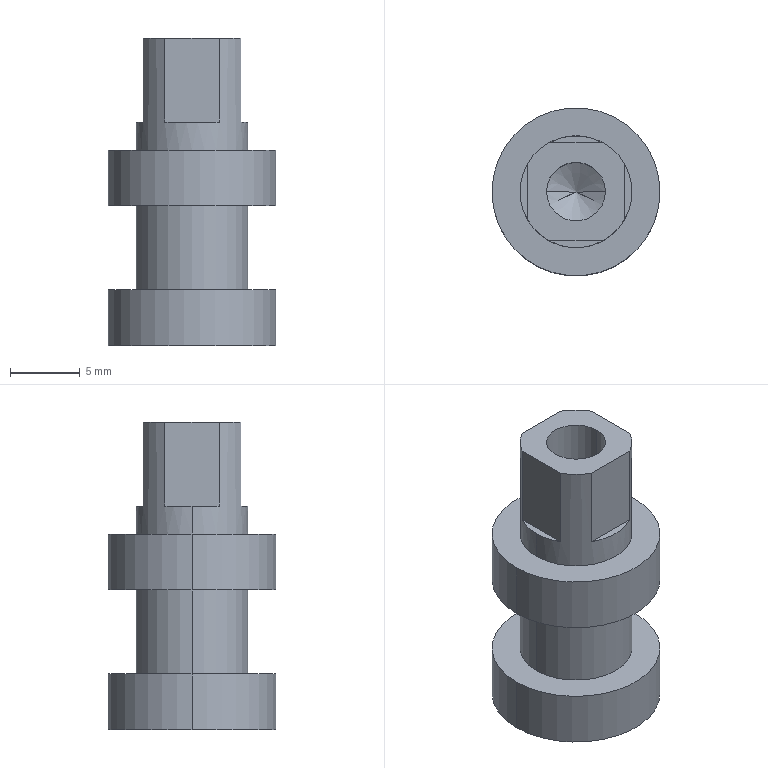Part | STEP file | Product shift T-head | 1 solid | 25 faces | box 12 x 12 x 22 mm | volume 1377 mm3 | plane 13 | cylinder 10 | cone 2 | commonest cylinder face diameters 8 x4 12 x4 4.2 x2